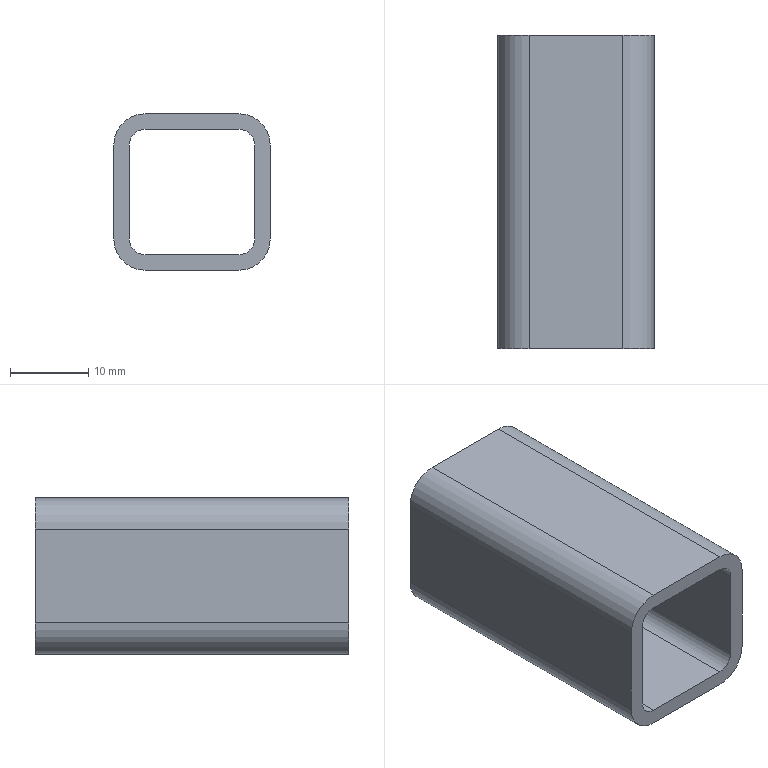Part | NX | features BREP 1 | 1 solid | 20 faces | box 20 x 40 x 20 mm | volume 5271 mm3 | cylinder 10 | plane 10 | commonest cylinder face diameters 4 x4 8 x4 7 x2
STEP:
#1=CARTESIAN_POINT('',(586.89,601.,1238.93));
#2=VERTEX_POINT('',#1);
#3=CARTESIAN_POINT('',(586.89,601.,1240.93));
#4=VERTEX_POINT('',#3);
#5=CARTESIAN_POINT('',(586.89,601.,1238.93));
#6=DIRECTION('',(0.,0.,1.));
#7=VECTOR('',#6,1000.);
#8=LINE('',#5,#7);
#9=EDGE_CURVE('',#2,#4,#8,.T.);
#10=ORIENTED_EDGE('',*,*,#9,.T.);
#11=CARTESIAN_POINT('',(593.89,601.,1240.93));
#12=VERTEX_POINT('',#11);
#13=CARTESIAN_POINT('',(590.39,601.,1240.93));
#14=DIRECTION('',(0.,0.,1.));
#15=DIRECTION('',(1.,0.,0.));
#16=AXIS2_PLACEMENT_3D('',#13,#14,#15);
#17=CIRCLE('',#16,3.5);
#18=EDGE_CURVE('',#4,#12,#17,.T.);
#19=ORIENTED_EDGE('',*,*,#18,.T.);
#20=CARTESIAN_POINT('',(593.89,601.,1238.93));
#21=VERTEX_POINT('',#20);
#22=CARTESIAN_POINT('',(593.89,601.,1238.93));
#23=DIRECTION('',(0.,0.,1.));
#24=VECTOR('',#23,1000.);
#25=LINE('',#22,#24);
#26=EDGE_CURVE('',#21,#12,#25,.T.);
#27=ORIENTED_EDGE('',*,*,#26,.F.);
#28=CARTESIAN_POINT('',(590.39,601.,1238.93));
#29=DIRECTION('',(0.,0.,1.));
#30=DIRECTION('',(1.,0.,0.));
#31=AXIS2_PLACEMENT_3D('',#28,#29,#30);
#32=CIRCLE('',#31,3.5);
#33=EDGE_CURVE('',#2,#21,#32,.T.);
#34=ORIENTED_EDGE('',*,*,#33,.F.);
#35=EDGE_LOOP('',(#10,#19,#27,#34));
#36=FACE_BOUND('',#35,.T.);
#37=CARTESIAN_POINT('',(590.39,601.,1238.93));
#38=DIRECTION('',(0.,0.,1.));
#39=DIRECTION('',(-1.,0.,0.));
#40=AXIS2_PLACEMENT_3D('',#37,#38,#39);
#41=CYLINDRICAL_SURFACE('',#40,3.5);
#42=ADVANCED_FACE('',(#36),#41,.F.);
#43=ORIENTED_EDGE('',*,*,#26,.T.);
#44=CARTESIAN_POINT('',(590.39,601.,1240.93));
#45=DIRECTION('',(0.,0.,1.));
#46=DIRECTION('',(1.,0.,0.));
#47=AXIS2_PLACEMENT_3D('',#44,#45,#46);
#48=CIRCLE('',#47,3.5);
#49=EDGE_CURVE('',#12,#4,#48,.T.);
#50=ORIENTED_EDGE('',*,*,#49,.T.);
#51=ORIENTED_EDGE('',*,*,#9,.F.);
#52=CARTESIAN_POINT('',(590.39,601.,1238.93));
#53=DIRECTION('',(0.,0.,1.));
#54=DIRECTION('',(1.,0.,0.));
#55=AXIS2_PLACEMENT_3D('',#52,#53,#54);
#56=CIRCLE('',#55,3.5);
#57=EDGE_CURVE('',#21,#2,#56,.T.);
#58=ORIENTED_EDGE('',*,*,#57,.F.);
#59=EDGE_LOOP('',(#43,#50,#51,#58));
#60=FACE_BOUND('',#59,.T.);
#61=CARTESIAN_POINT('',(590.39,601.,1238.93));
#62=DIRECTION('',(0.,0.,1.));
#63=DIRECTION('',(1.,0.,0.));
#64=AXIS2_PLACEMENT_3D('',#61,#62,#63);
#65=CYLINDRICAL_SURFACE('',#64,3.5);
#66=ADVANCED_FACE('',(#60),#65,.F.);
#67=CARTESIAN_POINT('',(598.387,621.,1254.93));
#68=VERTEX_POINT('',#67);
#69=CARTESIAN_POINT('',(598.387,621.,1242.93));
#70=VERTEX_POINT('',#69);
#71=CARTESIAN_POINT('',(598.387,621.,1248.93));
#72=DIRECTION('',(0.,0.,-1.));
#73=VECTOR('',#72,1000.);
#74=LINE('',#71,#73);
#75=EDGE_CURVE('',#68,#70,#74,.T.);
#76=ORIENTED_EDGE('',*,*,#75,.F.);
#77=CARTESIAN_POINT('',(596.387,621.,1256.93));
#78=VERTEX_POINT('',#77);
#79=CARTESIAN_POINT('',(596.387,621.,1254.93));
#80=DIRECTION('',(0.,-1.,0.));
#81=DIRECTION('',(1.,0.,0.));
#82=AXIS2_PLACEMENT_3D('',#79,#80,#81);
#83=CIRCLE('',#82,2.);
#84=EDGE_CURVE('',#68,#78,#83,.T.);
#85=ORIENTED_EDGE('',*,*,#84,.T.);
#86=CARTESIAN_POINT('',(584.387,621.,1256.93));
#87=VERTEX_POINT('',#86);
#88=CARTESIAN_POINT('',(590.387,621.,1256.93));
#89=DIRECTION('',(-1.,0.,0.));
#90=VECTOR('',#89,1000.);
#91=LINE('',#88,#90);
#92=EDGE_CURVE('',#78,#87,#91,.T.);
#93=ORIENTED_EDGE('',*,*,#92,.T.);
#94=CARTESIAN_POINT('',(582.387,621.,1254.93));
#95=VERTEX_POINT('',#94);
#96=CARTESIAN_POINT('',(584.387,621.,1254.93));
#97=DIRECTION('',(0.,-1.,0.));
#98=DIRECTION('',(1.,0.,0.));
#99=AXIS2_PLACEMENT_3D('',#96,#97,#98);
#100=CIRCLE('',#99,2.);
#101=EDGE_CURVE('',#87,#95,#100,.T.);
#102=ORIENTED_EDGE('',*,*,#101,.T.);
#103=CARTESIAN_POINT('',(582.387,621.,1242.93));
#104=VERTEX_POINT('',#103);
#105=CARTESIAN_POINT('',(582.387,621.,1248.93));
#106=DIRECTION('',(0.,0.,-1.));
#107=VECTOR('',#106,1000.);
#108=LINE('',#105,#107);
#109=EDGE_CURVE('',#95,#104,#108,.T.);
#110=ORIENTED_EDGE('',*,*,#109,.T.);
#111=CARTESIAN_POINT('',(584.387,621.,1240.93));
#112=VERTEX_POINT('',#111);
#113=CARTESIAN_POINT('',(584.387,621.,1242.93));
#114=DIRECTION('',(0.,-1.,0.));
#115=DIRECTION('',(1.,0.,0.));
#116=AXIS2_PLACEMENT_3D('',#113,#114,#115);
#117=CIRCLE('',#116,2.);
#118=EDGE_CURVE('',#104,#112,#117,.T.);
#119=ORIENTED_EDGE('',*,*,#118,.T.);
#120=CARTESIAN_POINT('',(596.387,621.,1240.93));
#121=VERTEX_POINT('',#120);
#122=CARTESIAN_POINT('',(590.387,621.,1240.93));
#123=DIRECTION('',(-1.,0.,0.));
#124=VECTOR('',#123,1000.);
#125=LINE('',#122,#124);
#126=EDGE_CURVE('',#121,#112,#125,.T.);
#127=ORIENTED_EDGE('',*,*,#126,.F.);
#128=CARTESIAN_POINT('',(596.387,621.,1242.93));
#129=DIRECTION('',(0.,-1.,0.));
#130=DIRECTION('',(1.,0.,0.));
#131=AXIS2_PLACEMENT_3D('',#128,#129,#130);
#132=CIRCLE('',#131,2.);
#133=EDGE_CURVE('',#121,#70,#132,.T.);
#134=ORIENTED_EDGE('',*,*,#133,.T.);
#135=EDGE_LOOP('',(#76,#85,#93,#102,#110,#119,#127,#134));
#136=FACE_BOUND('',#135,.T.);
#137=CARTESIAN_POINT('',(600.387,621.,1254.93));
#138=VERTEX_POINT('',#137);
#139=CARTESIAN_POINT('',(600.387,621.,1242.93));
#140=VERTEX_POINT('',#139);
#141=CARTESIAN_POINT('',(600.387,621.,1248.93));
#142=DIRECTION('',(0.,0.,-1.));
#143=VECTOR('',#142,1000.);
#144=LINE('',#141,#143);
#145=EDGE_CURVE('',#138,#140,#144,.T.);
#146=ORIENTED_EDGE('',*,*,#145,.T.);
#147=CARTESIAN_POINT('',(596.387,621.,1238.93));
#148=VERTEX_POINT('',#147);
#149=CARTESIAN_POINT('',(596.387,621.,1242.93));
#150=DIRECTION('',(0.,-1.,0.));
#151=DIRECTION('',(1.,0.,0.));
#152=AXIS2_PLACEMENT_3D('',#149,#150,#151);
#153=CIRCLE('',#152,4.);
#154=EDGE_CURVE('',#148,#140,#153,.T.);
#155=ORIENTED_EDGE('',*,*,#154,.F.);
#156=CARTESIAN_POINT('',(584.387,621.,1238.93));
#157=VERTEX_POINT('',#156);
#158=CARTESIAN_POINT('',(590.387,621.,1238.93));
#159=DIRECTION('',(-1.,0.,0.));
#160=VECTOR('',#159,1000.);
#161=LINE('',#158,#160);
#162=EDGE_CURVE('',#148,#157,#161,.T.);
#163=ORIENTED_EDGE('',*,*,#162,.T.);
#164=CARTESIAN_POINT('',(580.387,621.,1242.93));
#165=VERTEX_POINT('',#164);
#166=CARTESIAN_POINT('',(584.387,621.,1242.93));
#167=DIRECTION('',(0.,-1.,0.));
#168=DIRECTION('',(1.,0.,0.));
#169=AXIS2_PLACEMENT_3D('',#166,#167,#168);
#170=CIRCLE('',#169,4.);
#171=EDGE_CURVE('',#165,#157,#170,.T.);
#172=ORIENTED_EDGE('',*,*,#171,.F.);
#173=CARTESIAN_POINT('',(580.387,621.,1254.93));
#174=VERTEX_POINT('',#173);
#175=CARTESIAN_POINT('',(580.387,621.,1248.93));
#176=DIRECTION('',(0.,0.,-1.));
#177=VECTOR('',#176,1000.);
#178=LINE('',#175,#177);
#179=EDGE_CURVE('',#174,#165,#178,.T.);
#180=ORIENTED_EDGE('',*,*,#179,.F.);
#181=CARTESIAN_POINT('',(584.387,621.,1258.93));
#182=VERTEX_POINT('',#181);
#183=CARTESIAN_POINT('',(584.387,621.,1254.93));
#184=DIRECTION('',(0.,-1.,0.));
#185=DIRECTION('',(1.,0.,0.));
#186=AXIS2_PLACEMENT_3D('',#183,#184,#185);
#187=CIRCLE('',#186,4.);
#188=EDGE_CURVE('',#182,#174,#187,.T.);
#189=ORIENTED_EDGE('',*,*,#188,.F.);
#190=CARTESIAN_POINT('',(596.387,621.,1258.93));
#191=VERTEX_POINT('',#190);
#192=CARTESIAN_POINT('',(590.387,621.,1258.93));
#193=DIRECTION('',(-1.,0.,0.));
#194=VECTOR('',#193,1000.);
#195=LINE('',#192,#194);
#196=EDGE_CURVE('',#191,#182,#195,.T.);
#197=ORIENTED_EDGE('',*,*,#196,.F.);
#198=CARTESIAN_POINT('',(596.387,621.,1254.93));
#199=DIRECTION('',(0.,-1.,0.));
#200=DIRECTION('',(1.,0.,0.));
#201=AXIS2_PLACEMENT_3D('',#198,#199,#200);
#202=CIRCLE('',#201,4.);
#203=EDGE_CURVE('',#138,#191,#202,.T.);
#204=ORIENTED_EDGE('',*,*,#203,.F.);
#205=EDGE_LOOP('',(#146,#155,#163,#172,#180,#189,#197,#204));
#206=FACE_BOUND('',#205,.T.);
#207=CARTESIAN_POINT('',(603.464,621.,1238.93));
#208=DIRECTION('',(0.,-1.,0.));
#209=DIRECTION('',(-1.,0.,0.));
#210=AXIS2_PLACEMENT_3D('',#207,#208,#209);
#211=PLANE('',#210);
#212=ADVANCED_FACE('',(#136,#206),#211,.F.);
#213=CARTESIAN_POINT('',(596.387,581.,1256.93));
#214=VERTEX_POINT('',#213);
#215=CARTESIAN_POINT('',(596.387,601.,1256.93));
#216=DIRECTION('',(0.,-1.,0.));
#217=VECTOR('',#216,1000.);
#218=LINE('',#215,#217);
#219=EDGE_CURVE('',#78,#214,#218,.T.);
#220=ORIENTED_EDGE('',*,*,#219,.F.);
#221=ORIENTED_EDGE('',*,*,#84,.F.);
#222=CARTESIAN_POINT('',(598.387,581.,1254.93));
#223=VERTEX_POINT('',#222);
#224=CARTESIAN_POINT('',(598.387,601.,1254.93));
#225=DIRECTION('',(0.,-1.,0.));
#226=VECTOR('',#225,1000.);
#227=LINE('',#224,#226);
#228=EDGE_CURVE('',#68,#223,#227,.T.);
#229=ORIENTED_EDGE('',*,*,#228,.T.);
#230=CARTESIAN_POINT('',(596.387,581.,1254.93));
#231=DIRECTION('',(0.,1.,0.));
#232=DIRECTION('',(1.,0.,0.));
#233=AXIS2_PLACEMENT_3D('',#230,#231,#232);
#234=CIRCLE('',#233,2.);
#235=EDGE_CURVE('',#214,#223,#234,.T.);
#236=ORIENTED_EDGE('',*,*,#235,.F.);
#237=EDGE_LOOP('',(#220,#221,#229,#236));
#238=FACE_BOUND('',#237,.T.);
#239=CARTESIAN_POINT('',(596.387,-597.81,1254.93));
#240=DIRECTION('',(0.,-1.,0.));
#241=DIRECTION('',(1.,0.,0.));
#242=AXIS2_PLACEMENT_3D('',#239,#240,#241);
#243=CYLINDRICAL_SURFACE('',#242,2.);
#244=ADVANCED_FACE('',(#238),#243,.F.);
#245=CARTESIAN_POINT('',(584.387,581.,1256.93));
#246=VERTEX_POINT('',#245);
#247=CARTESIAN_POINT('',(590.387,581.,1256.93));
#248=DIRECTION('',(-1.,0.,0.));
#249=VECTOR('',#248,1000.);
#250=LINE('',#247,#249);
#251=EDGE_CURVE('',#214,#246,#250,.T.);
#252=ORIENTED_EDGE('',*,*,#251,.T.);
#253=CARTESIAN_POINT('',(584.387,-597.81,1256.93));
#254=DIRECTION('',(0.,-1.,0.));
#255=VECTOR('',#254,1000.);
#256=LINE('',#253,#255);
#257=EDGE_CURVE('',#87,#246,#256,.T.);
#258=ORIENTED_EDGE('',*,*,#257,.F.);
#259=ORIENTED_EDGE('',*,*,#92,.F.);
#260=ORIENTED_EDGE('',*,*,#219,.T.);
#261=EDGE_LOOP('',(#252,#258,#259,#260));
#262=FACE_BOUND('',#261,.T.);
#263=CARTESIAN_POINT('',(596.387,-597.81,1256.93));
#264=DIRECTION('',(0.,0.,-1.));
#265=DIRECTION('',(0.,1.,0.));
#266=AXIS2_PLACEMENT_3D('',#263,#264,#265);
#267=PLANE('',#266);
#268=ADVANCED_FACE('',(#262),#267,.T.);
#269=CARTESIAN_POINT('',(582.387,581.,1254.93));
#270=VERTEX_POINT('',#269);
#271=CARTESIAN_POINT('',(582.387,601.,1254.93));
#272=DIRECTION('',(0.,-1.,0.));
#273=VECTOR('',#272,1000.);
#274=LINE('',#271,#273);
#275=EDGE_CURVE('',#95,#270,#274,.T.);
#276=ORIENTED_EDGE('',*,*,#275,.F.);
#277=ORIENTED_EDGE('',*,*,#101,.F.);
#278=ORIENTED_EDGE('',*,*,#257,.T.);
#279=CARTESIAN_POINT('',(584.387,581.,1254.93));
#280=DIRECTION('',(0.,1.,0.));
#281=DIRECTION('',(1.,0.,0.));
#282=AXIS2_PLACEMENT_3D('',#279,#280,#281);
#283=CIRCLE('',#282,2.);
#284=EDGE_CURVE('',#270,#246,#283,.T.);
#285=ORIENTED_EDGE('',*,*,#284,.F.);
#286=EDGE_LOOP('',(#276,#277,#278,#285));
#287=FACE_BOUND('',#286,.T.);
#288=CARTESIAN_POINT('',(584.387,-597.81,1254.93));
#289=DIRECTION('',(0.,-1.,0.));
#290=DIRECTION('',(1.,0.,0.));
#291=AXIS2_PLACEMENT_3D('',#288,#289,#290);
#292=CYLINDRICAL_SURFACE('',#291,2.);
#293=ADVANCED_FACE('',(#287),#292,.F.);
#294=CARTESIAN_POINT('',(582.387,581.,1242.93));
#295=VERTEX_POINT('',#294);
#296=CARTESIAN_POINT('',(582.387,581.,1248.93));
#297=DIRECTION('',(0.,0.,-1.));
#298=VECTOR('',#297,1000.);
#299=LINE('',#296,#298);
#300=EDGE_CURVE('',#270,#295,#299,.T.);
#301=ORIENTED_EDGE('',*,*,#300,.T.);
#302=CARTESIAN_POINT('',(582.387,-597.81,1242.93));
#303=DIRECTION('',(0.,-1.,0.));
#304=VECTOR('',#303,1000.);
#305=LINE('',#302,#304);
#306=EDGE_CURVE('',#104,#295,#305,.T.);
#307=ORIENTED_EDGE('',*,*,#306,.F.);
#308=ORIENTED_EDGE('',*,*,#109,.F.);
#309=ORIENTED_EDGE('',*,*,#275,.T.);
#310=EDGE_LOOP('',(#301,#307,#308,#309));
#311=FACE_BOUND('',#310,.T.);
#312=CARTESIAN_POINT('',(582.387,-597.81,1254.93));
#313=DIRECTION('',(1.,0.,0.));
#314=DIRECTION('',(0.,1.,0.));
#315=AXIS2_PLACEMENT_3D('',#312,#313,#314);
#316=PLANE('',#315);
#317=ADVANCED_FACE('',(#311),#316,.T.);
#318=CARTESIAN_POINT('',(584.387,581.,1240.93));
#319=VERTEX_POINT('',#318);
#320=CARTESIAN_POINT('',(584.387,601.,1240.93));
#321=DIRECTION('',(0.,-1.,0.));
#322=VECTOR('',#321,1000.);
#323=LINE('',#320,#322);
#324=EDGE_CURVE('',#112,#319,#323,.T.);
#325=ORIENTED_EDGE('',*,*,#324,.F.);
#326=ORIENTED_EDGE('',*,*,#118,.F.);
#327=ORIENTED_EDGE('',*,*,#306,.T.);
#328=CARTESIAN_POINT('',(584.387,581.,1242.93));
#329=DIRECTION('',(0.,1.,0.));
#330=DIRECTION('',(1.,0.,0.));
#331=AXIS2_PLACEMENT_3D('',#328,#329,#330);
#332=CIRCLE('',#331,2.);
#333=EDGE_CURVE('',#319,#295,#332,.T.);
#334=ORIENTED_EDGE('',*,*,#333,.F.);
#335=EDGE_LOOP('',(#325,#326,#327,#334));
#336=FACE_BOUND('',#335,.T.);
#337=CARTESIAN_POINT('',(584.387,-597.81,1242.93));
#338=DIRECTION('',(0.,-1.,0.));
#339=DIRECTION('',(-1.,0.,0.));
#340=AXIS2_PLACEMENT_3D('',#337,#338,#339);
#341=CYLINDRICAL_SURFACE('',#340,2.);
#342=ADVANCED_FACE('',(#336),#341,.F.);
#343=ORIENTED_EDGE('',*,*,#18,.F.);
#344=ORIENTED_EDGE('',*,*,#49,.F.);
#345=EDGE_LOOP('',(#343,#344));
#346=FACE_BOUND('',#345,.T.);
#347=CARTESIAN_POINT('',(596.387,581.,1240.93));
#348=VERTEX_POINT('',#347);
#349=CARTESIAN_POINT('',(590.387,581.,1240.93));
#350=DIRECTION('',(-1.,0.,0.));
#351=VECTOR('',#350,1000.);
#352=LINE('',#349,#351);
#353=EDGE_CURVE('',#348,#319,#352,.T.);
#354=ORIENTED_EDGE('',*,*,#353,.F.);
#355=CARTESIAN_POINT('',(596.387,-597.81,1240.93));
#356=DIRECTION('',(0.,-1.,0.));
#357=VECTOR('',#356,1000.);
#358=LINE('',#355,#357);
#359=EDGE_CURVE('',#121,#348,#358,.T.);
#360=ORIENTED_EDGE('',*,*,#359,.F.);
#361=ORIENTED_EDGE('',*,*,#126,.T.);
#362=ORIENTED_EDGE('',*,*,#324,.T.);
#363=EDGE_LOOP('',(#354,#360,#361,#362));
#364=FACE_BOUND('',#363,.T.);
#365=CARTESIAN_POINT('',(584.387,-597.81,1240.93));
#366=DIRECTION('',(0.,0.,1.));
#367=DIRECTION('',(0.,-1.,0.));
#368=AXIS2_PLACEMENT_3D('',#365,#366,#367);
#369=PLANE('',#368);
#370=ADVANCED_FACE('',(#346,#364),#369,.T.);
#371=CARTESIAN_POINT('',(598.387,581.,1242.93));
#372=VERTEX_POINT('',#371);
#373=CARTESIAN_POINT('',(598.387,601.,1242.93));
#374=DIRECTION('',(0.,-1.,0.));
#375=VECTOR('',#374,1000.);
#376=LINE('',#373,#375);
#377=EDGE_CURVE('',#70,#372,#376,.T.);
#378=ORIENTED_EDGE('',*,*,#377,.F.);
#379=ORIENTED_EDGE('',*,*,#133,.F.);
#380=ORIENTED_EDGE('',*,*,#359,.T.);
#381=CARTESIAN_POINT('',(596.387,581.,1242.93));
#382=DIRECTION('',(0.,1.,0.));
#383=DIRECTION('',(1.,0.,0.));
#384=AXIS2_PLACEMENT_3D('',#381,#382,#383);
#385=CIRCLE('',#384,2.);
#386=EDGE_CURVE('',#372,#348,#385,.T.);
#387=ORIENTED_EDGE('',*,*,#386,.F.);
#388=EDGE_LOOP('',(#378,#379,#380,#387));
#389=FACE_BOUND('',#388,.T.);
#390=CARTESIAN_POINT('',(596.387,-597.81,1242.93));
#391=DIRECTION('',(0.,-1.,0.));
#392=DIRECTION('',(-1.,0.,0.));
#393=AXIS2_PLACEMENT_3D('',#390,#391,#392);
#394=CYLINDRICAL_SURFACE('',#393,2.);
#395=ADVANCED_FACE('',(#389),#394,.F.);
#396=ORIENTED_EDGE('',*,*,#228,.F.);
#397=ORIENTED_EDGE('',*,*,#75,.T.);
#398=ORIENTED_EDGE('',*,*,#377,.T.);
#399=CARTESIAN_POINT('',(598.387,581.,1248.93));
#400=DIRECTION('',(0.,0.,-1.));
#401=VECTOR('',#400,1000.);
#402=LINE('',#399,#401);
#403=EDGE_CURVE('',#223,#372,#402,.T.);
#404=ORIENTED_EDGE('',*,*,#403,.F.);
#405=EDGE_LOOP('',(#396,#397,#398,#404));
#406=FACE_BOUND('',#405,.T.);
#407=CARTESIAN_POINT('',(598.387,-597.81,1242.93));
#408=DIRECTION('',(-1.,0.,0.));
#409=DIRECTION('',(0.,-1.,0.));
#410=AXIS2_PLACEMENT_3D('',#407,#408,#409);
#411=PLANE('',#410);
#412=ADVANCED_FACE('',(#406),#411,.T.);
#413=CARTESIAN_POINT('',(600.387,581.,1242.93));
#414=VERTEX_POINT('',#413);
#415=CARTESIAN_POINT('',(596.387,581.,1238.93));
#416=VERTEX_POINT('',#415);
#417=CARTESIAN_POINT('',(596.387,581.,1242.93));
#418=DIRECTION('',(0.,1.,0.));
#419=DIRECTION('',(1.,0.,0.));
#420=AXIS2_PLACEMENT_3D('',#417,#418,#419);
#421=CIRCLE('',#420,4.);
#422=EDGE_CURVE('',#414,#416,#421,.T.);
#423=ORIENTED_EDGE('',*,*,#422,.T.);
#424=CARTESIAN_POINT('',(596.387,601.,1238.93));
#425=DIRECTION('',(0.,-1.,0.));
#426=VECTOR('',#425,1000.);
#427=LINE('',#424,#426);
#428=EDGE_CURVE('',#148,#416,#427,.T.);
#429=ORIENTED_EDGE('',*,*,#428,.F.);
#430=ORIENTED_EDGE('',*,*,#154,.T.);
#431=CARTESIAN_POINT('',(600.387,601.,1242.93));
#432=DIRECTION('',(0.,-1.,0.));
#433=VECTOR('',#432,1000.);
#434=LINE('',#431,#433);
#435=EDGE_CURVE('',#140,#414,#434,.T.);
#436=ORIENTED_EDGE('',*,*,#435,.T.);
#437=EDGE_LOOP('',(#423,#429,#430,#436));
#438=FACE_BOUND('',#437,.T.);
#439=CARTESIAN_POINT('',(596.387,-597.81,1242.93));
#440=DIRECTION('',(0.,-1.,0.));
#441=DIRECTION('',(-1.,0.,0.));
#442=AXIS2_PLACEMENT_3D('',#439,#440,#441);
#443=CYLINDRICAL_SURFACE('',#442,4.);
#444=ADVANCED_FACE('',(#438),#443,.T.);
#445=ORIENTED_EDGE('',*,*,#57,.T.);
#446=ORIENTED_EDGE('',*,*,#33,.T.);
#447=EDGE_LOOP('',(#445,#446));
#448=FACE_BOUND('',#447,.T.);
#449=CARTESIAN_POINT('',(584.387,581.,1238.93));
#450=VERTEX_POINT('',#449);
#451=CARTESIAN_POINT('',(584.387,-597.81,1238.93));
#452=DIRECTION('',(0.,-1.,0.));
#453=VECTOR('',#452,1000.);
#454=LINE('',#451,#453);
#455=EDGE_CURVE('',#157,#450,#454,.T.);
#456=ORIENTED_EDGE('',*,*,#455,.F.);
#457=ORIENTED_EDGE('',*,*,#162,.F.);
#458=ORIENTED_EDGE('',*,*,#428,.T.);
#459=CARTESIAN_POINT('',(590.387,581.,1238.93));
#460=DIRECTION('',(-1.,0.,0.));
#461=VECTOR('',#460,1000.);
#462=LINE('',#459,#461);
#463=EDGE_CURVE('',#416,#450,#462,.T.);
#464=ORIENTED_EDGE('',*,*,#463,.T.);
#465=EDGE_LOOP('',(#456,#457,#458,#464));
#466=FACE_BOUND('',#465,.T.);
#467=CARTESIAN_POINT('',(584.387,-597.81,1238.93));
#468=DIRECTION('',(0.,0.,1.));
#469=DIRECTION('',(0.,-1.,0.));
#470=AXIS2_PLACEMENT_3D('',#467,#468,#469);
#471=PLANE('',#470);
#472=ADVANCED_FACE('',(#448,#466),#471,.F.);
#473=CARTESIAN_POINT('',(580.387,581.,1242.93));
#474=VERTEX_POINT('',#473);
#475=CARTESIAN_POINT('',(584.387,581.,1242.93));
#476=DIRECTION('',(0.,1.,0.));
#477=DIRECTION('',(1.,0.,0.));
#478=AXIS2_PLACEMENT_3D('',#475,#476,#477);
#479=CIRCLE('',#478,4.);
#480=EDGE_CURVE('',#450,#474,#479,.T.);
#481=ORIENTED_EDGE('',*,*,#480,.T.);
#482=CARTESIAN_POINT('',(580.387,601.,1242.93));
#483=DIRECTION('',(0.,-1.,0.));
#484=VECTOR('',#483,1000.);
#485=LINE('',#482,#484);
#486=EDGE_CURVE('',#165,#474,#485,.T.);
#487=ORIENTED_EDGE('',*,*,#486,.F.);
#488=ORIENTED_EDGE('',*,*,#171,.T.);
#489=ORIENTED_EDGE('',*,*,#455,.T.);
#490=EDGE_LOOP('',(#481,#487,#488,#489));
#491=FACE_BOUND('',#490,.T.);
#492=CARTESIAN_POINT('',(584.387,-597.81,1242.93));
#493=DIRECTION('',(0.,-1.,0.));
#494=DIRECTION('',(-1.,0.,0.));
#495=AXIS2_PLACEMENT_3D('',#492,#493,#494);
#496=CYLINDRICAL_SURFACE('',#495,4.);
#497=ADVANCED_FACE('',(#491),#496,.T.);
#498=CARTESIAN_POINT('',(580.387,581.,1254.93));
#499=VERTEX_POINT('',#498);
#500=CARTESIAN_POINT('',(580.387,-597.81,1254.93));
#501=DIRECTION('',(0.,-1.,0.));
#502=VECTOR('',#501,1000.);
#503=LINE('',#500,#502);
#504=EDGE_CURVE('',#174,#499,#503,.T.);
#505=ORIENTED_EDGE('',*,*,#504,.F.);
#506=ORIENTED_EDGE('',*,*,#179,.T.);
#507=ORIENTED_EDGE('',*,*,#486,.T.);
#508=CARTESIAN_POINT('',(580.387,581.,1248.93));
#509=DIRECTION('',(0.,0.,-1.));
#510=VECTOR('',#509,1000.);
#511=LINE('',#508,#510);
#512=EDGE_CURVE('',#499,#474,#511,.T.);
#513=ORIENTED_EDGE('',*,*,#512,.F.);
#514=EDGE_LOOP('',(#505,#506,#507,#513));
#515=FACE_BOUND('',#514,.T.);
#516=CARTESIAN_POINT('',(580.387,-597.81,1254.93));
#517=DIRECTION('',(1.,0.,0.));
#518=DIRECTION('',(0.,1.,0.));
#519=AXIS2_PLACEMENT_3D('',#516,#517,#518);
#520=PLANE('',#519);
#521=ADVANCED_FACE('',(#515),#520,.F.);
#522=CARTESIAN_POINT('',(584.387,581.,1258.93));
#523=VERTEX_POINT('',#522);
#524=CARTESIAN_POINT('',(584.387,581.,1254.93));
#525=DIRECTION('',(0.,1.,0.));
#526=DIRECTION('',(1.,0.,0.));
#527=AXIS2_PLACEMENT_3D('',#524,#525,#526);
#528=CIRCLE('',#527,4.);
#529=EDGE_CURVE('',#499,#523,#528,.T.);
#530=ORIENTED_EDGE('',*,*,#529,.T.);
#531=CARTESIAN_POINT('',(584.387,601.,1258.93));
#532=DIRECTION('',(0.,-1.,0.));
#533=VECTOR('',#532,1000.);
#534=LINE('',#531,#533);
#535=EDGE_CURVE('',#182,#523,#534,.T.);
#536=ORIENTED_EDGE('',*,*,#535,.F.);
#537=ORIENTED_EDGE('',*,*,#188,.T.);
#538=ORIENTED_EDGE('',*,*,#504,.T.);
#539=EDGE_LOOP('',(#530,#536,#537,#538));
#540=FACE_BOUND('',#539,.T.);
#541=CARTESIAN_POINT('',(584.387,-597.81,1254.93));
#542=DIRECTION('',(0.,-1.,0.));
#543=DIRECTION('',(1.,0.,0.));
#544=AXIS2_PLACEMENT_3D('',#541,#542,#543);
#545=CYLINDRICAL_SURFACE('',#544,4.);
#546=ADVANCED_FACE('',(#540),#545,.T.);
#547=CARTESIAN_POINT('',(596.387,581.,1258.93));
#548=VERTEX_POINT('',#547);
#549=CARTESIAN_POINT('',(596.387,-597.81,1258.93));
#550=DIRECTION('',(0.,-1.,0.));
#551=VECTOR('',#550,1000.);
#552=LINE('',#549,#551);
#553=EDGE_CURVE('',#191,#548,#552,.T.);
#554=ORIENTED_EDGE('',*,*,#553,.F.);
#555=ORIENTED_EDGE('',*,*,#196,.T.);
#556=ORIENTED_EDGE('',*,*,#535,.T.);
#557=CARTESIAN_POINT('',(590.387,581.,1258.93));
#558=DIRECTION('',(-1.,0.,0.));
#559=VECTOR('',#558,1000.);
#560=LINE('',#557,#559);
#561=EDGE_CURVE('',#548,#523,#560,.T.);
#562=ORIENTED_EDGE('',*,*,#561,.F.);
#563=EDGE_LOOP('',(#554,#555,#556,#562));
#564=FACE_BOUND('',#563,.T.);
#565=CARTESIAN_POINT('',(596.387,-597.81,1258.93));
#566=DIRECTION('',(0.,0.,-1.));
#567=DIRECTION('',(0.,1.,0.));
#568=AXIS2_PLACEMENT_3D('',#565,#566,#567);
#569=PLANE('',#568);
#570=ADVANCED_FACE('',(#564),#569,.F.);
#571=CARTESIAN_POINT('',(600.387,581.,1254.93));
#572=VERTEX_POINT('',#571);
#573=CARTESIAN_POINT('',(596.387,581.,1254.93));
#574=DIRECTION('',(0.,1.,0.));
#575=DIRECTION('',(1.,0.,0.));
#576=AXIS2_PLACEMENT_3D('',#573,#574,#575);
#577=CIRCLE('',#576,4.);
#578=EDGE_CURVE('',#548,#572,#577,.T.);
#579=ORIENTED_EDGE('',*,*,#578,.T.);
#580=CARTESIAN_POINT('',(600.387,601.,1254.93));
#581=DIRECTION('',(0.,-1.,0.));
#582=VECTOR('',#581,1000.);
#583=LINE('',#580,#582);
#584=EDGE_CURVE('',#138,#572,#583,.T.);
#585=ORIENTED_EDGE('',*,*,#584,.F.);
#586=ORIENTED_EDGE('',*,*,#203,.T.);
#587=ORIENTED_EDGE('',*,*,#553,.T.);
#588=EDGE_LOOP('',(#579,#585,#586,#587));
#589=FACE_BOUND('',#588,.T.);
#590=CARTESIAN_POINT('',(596.387,-597.81,1254.93));
#591=DIRECTION('',(0.,-1.,0.));
#592=DIRECTION('',(1.,0.,0.));
#593=AXIS2_PLACEMENT_3D('',#590,#591,#592);
#594=CYLINDRICAL_SURFACE('',#593,4.);
#595=ADVANCED_FACE('',(#589),#594,.T.);
#596=ORIENTED_EDGE('',*,*,#584,.T.);
#597=CARTESIAN_POINT('',(600.387,581.,1248.93));
#598=DIRECTION('',(0.,0.,-1.));
#599=VECTOR('',#598,1000.);
#600=LINE('',#597,#599);
#601=EDGE_CURVE('',#572,#414,#600,.T.);
#602=ORIENTED_EDGE('',*,*,#601,.T.);
#603=ORIENTED_EDGE('',*,*,#435,.F.);
#604=ORIENTED_EDGE('',*,*,#145,.F.);
#605=EDGE_LOOP('',(#596,#602,#603,#604));
#606=FACE_BOUND('',#605,.T.);
#607=CARTESIAN_POINT('',(600.387,-597.81,1242.93));
#608=DIRECTION('',(-1.,0.,0.));
#609=DIRECTION('',(0.,-1.,0.));
#610=AXIS2_PLACEMENT_3D('',#607,#608,#609);
#611=PLANE('',#610);
#612=ADVANCED_FACE('',(#606),#611,.F.);
#613=ORIENTED_EDGE('',*,*,#403,.T.);
#614=ORIENTED_EDGE('',*,*,#386,.T.);
#615=ORIENTED_EDGE('',*,*,#353,.T.);
#616=ORIENTED_EDGE('',*,*,#333,.T.);
#617=ORIENTED_EDGE('',*,*,#300,.F.);
#618=ORIENTED_EDGE('',*,*,#284,.T.);
#619=ORIENTED_EDGE('',*,*,#251,.F.);
#620=ORIENTED_EDGE('',*,*,#235,.T.);
#621=EDGE_LOOP('',(#613,#614,#615,#616,#617,#618,#619,#620));
#622=FACE_BOUND('',#621,.T.);
#623=ORIENTED_EDGE('',*,*,#601,.F.);
#624=ORIENTED_EDGE('',*,*,#578,.F.);
#625=ORIENTED_EDGE('',*,*,#561,.T.);
#626=ORIENTED_EDGE('',*,*,#529,.F.);
#627=ORIENTED_EDGE('',*,*,#512,.T.);
#628=ORIENTED_EDGE('',*,*,#480,.F.);
#629=ORIENTED_EDGE('',*,*,#463,.F.);
#630=ORIENTED_EDGE('',*,*,#422,.F.);
#631=EDGE_LOOP('',(#623,#624,#625,#626,#627,#628,#629,#630));
#632=FACE_BOUND('',#631,.T.);
#633=CARTESIAN_POINT('',(577.316,581.,1238.93));
#634=DIRECTION('',(0.,1.,0.));
#635=DIRECTION('',(1.,0.,0.));
#636=AXIS2_PLACEMENT_3D('',#633,#634,#635);
#637=PLANE('',#636);
#638=ADVANCED_FACE('',(#622,#632),#637,.F.);
#639=CLOSED_SHELL('',(#42,#66,#212,#244,#268,#293,#317,#342,#370,#395,#412,#444,#472,#497,#521,#546,#570,#595,#612,#638));
#640=MANIFOLD_SOLID_BREP('',#639);
#641=(LENGTH_UNIT()NAMED_UNIT(*)SI_UNIT(.MILLI.,.METRE.));
#642=UNCERTAINTY_MEASURE_WITH_UNIT(LENGTH_MEASURE(0.00001),#641,'','');
#643=(NAMED_UNIT(*)PLANE_ANGLE_UNIT()SI_UNIT($,.RADIAN.));
#644=(NAMED_UNIT(*)SI_UNIT($,.STERADIAN.)SOLID_ANGLE_UNIT());
#645=(GEOMETRIC_REPRESENTATION_CONTEXT(3)GLOBAL_UNCERTAINTY_ASSIGNED_CONTEXT((#642))GLOBAL_UNIT_ASSIGNED_CONTEXT((#641,#643,#644))REPRESENTATION_CONTEXT('',''));
#646=ADVANCED_BREP_SHAPE_REPRESENTATION('',(#640),#645);